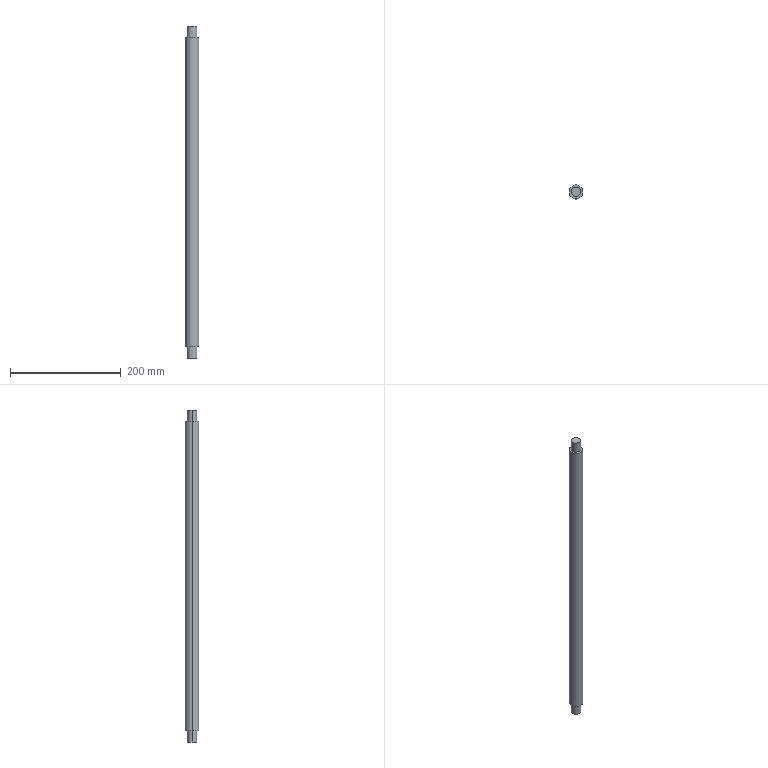Part | SolidWorks | features BaseBody 1 | 1 solid | 10 faces | box 25 x 25 x 600 mm | volume 283969 mm3 | cylinder 6 | plane 4 | commonest cylinder face diameters 17 x4 25 x2
STEP:
#1=CARTESIAN_POINT('',(8.5,0.,-560.));
#2=VERTEX_POINT('',#1);
#3=CARTESIAN_POINT('',(-8.5,0.,-560.));
#4=VERTEX_POINT('',#3);
#5=CARTESIAN_POINT('',(0.,0.,-560.));
#6=DIRECTION('',(0.,0.,1.));
#7=DIRECTION('',(-1.,0.,0.));
#8=AXIS2_PLACEMENT_3D('',#5,#6,#7);
#9=CIRCLE('',#8,8.5);
#10=EDGE_CURVE('',#2,#4,#9,.T.);
#11=ORIENTED_EDGE('',*,*,#10,.F.);
#12=CARTESIAN_POINT('',(8.5,0.,-580.));
#13=VERTEX_POINT('',#12);
#14=CARTESIAN_POINT('',(8.5,0.,-580.));
#15=DIRECTION('',(0.,0.,-1.));
#16=VECTOR('',#15,1000.);
#17=LINE('',#14,#16);
#18=EDGE_CURVE('',#2,#13,#17,.T.);
#19=ORIENTED_EDGE('',*,*,#18,.T.);
#20=CARTESIAN_POINT('',(-8.5,0.,-580.));
#21=VERTEX_POINT('',#20);
#22=CARTESIAN_POINT('',(0.,0.,-580.));
#23=DIRECTION('',(0.,0.,-1.));
#24=DIRECTION('',(-1.,0.,0.));
#25=AXIS2_PLACEMENT_3D('',#22,#23,#24);
#26=CIRCLE('',#25,8.5);
#27=EDGE_CURVE('',#21,#13,#26,.T.);
#28=ORIENTED_EDGE('',*,*,#27,.F.);
#29=CARTESIAN_POINT('',(-8.5,0.,-580.));
#30=DIRECTION('',(0.,0.,-1.));
#31=VECTOR('',#30,1000.);
#32=LINE('',#29,#31);
#33=EDGE_CURVE('',#4,#21,#32,.T.);
#34=ORIENTED_EDGE('',*,*,#33,.F.);
#35=EDGE_LOOP('',(#11,#19,#28,#34));
#36=FACE_OUTER_BOUND('',#35,.T.);
#37=CARTESIAN_POINT('',(0.,0.,-580.));
#38=DIRECTION('',(0.,0.,-1.));
#39=DIRECTION('',(-1.,0.,0.));
#40=AXIS2_PLACEMENT_3D('',#37,#38,#39);
#41=CYLINDRICAL_SURFACE('',#40,8.5);
#42=ADVANCED_FACE('',(#36),#41,.T.);
#43=CARTESIAN_POINT('',(8.5,0.,20.));
#44=VERTEX_POINT('',#43);
#45=CARTESIAN_POINT('',(-8.5,0.,20.));
#46=VERTEX_POINT('',#45);
#47=CARTESIAN_POINT('',(0.,0.,20.));
#48=DIRECTION('',(0.,0.,1.));
#49=DIRECTION('',(-1.,0.,0.));
#50=AXIS2_PLACEMENT_3D('',#47,#48,#49);
#51=CIRCLE('',#50,8.5);
#52=EDGE_CURVE('',#44,#46,#51,.T.);
#53=ORIENTED_EDGE('',*,*,#52,.F.);
#54=CARTESIAN_POINT('',(8.5,0.,0.));
#55=VERTEX_POINT('',#54);
#56=CARTESIAN_POINT('',(8.5,0.,0.));
#57=DIRECTION('',(0.,0.,-1.));
#58=VECTOR('',#57,1000.);
#59=LINE('',#56,#58);
#60=EDGE_CURVE('',#44,#55,#59,.T.);
#61=ORIENTED_EDGE('',*,*,#60,.T.);
#62=CARTESIAN_POINT('',(-8.5,0.,0.));
#63=VERTEX_POINT('',#62);
#64=CARTESIAN_POINT('',(0.,0.,0.));
#65=DIRECTION('',(0.,0.,-1.));
#66=DIRECTION('',(-1.,0.,0.));
#67=AXIS2_PLACEMENT_3D('',#64,#65,#66);
#68=CIRCLE('',#67,8.5);
#69=EDGE_CURVE('',#63,#55,#68,.T.);
#70=ORIENTED_EDGE('',*,*,#69,.F.);
#71=CARTESIAN_POINT('',(-8.5,0.,0.));
#72=DIRECTION('',(0.,0.,-1.));
#73=VECTOR('',#72,1000.);
#74=LINE('',#71,#73);
#75=EDGE_CURVE('',#46,#63,#74,.T.);
#76=ORIENTED_EDGE('',*,*,#75,.F.);
#77=EDGE_LOOP('',(#53,#61,#70,#76));
#78=FACE_OUTER_BOUND('',#77,.T.);
#79=CARTESIAN_POINT('',(0.,0.,0.));
#80=DIRECTION('',(0.,0.,-1.));
#81=DIRECTION('',(-1.,0.,0.));
#82=AXIS2_PLACEMENT_3D('',#79,#80,#81);
#83=CYLINDRICAL_SURFACE('',#82,8.5);
#84=ADVANCED_FACE('',(#78),#83,.T.);
#85=CARTESIAN_POINT('',(12.5,0.,-560.));
#86=VERTEX_POINT('',#85);
#87=CARTESIAN_POINT('',(-12.5,0.,-560.));
#88=VERTEX_POINT('',#87);
#89=CARTESIAN_POINT('',(0.,0.,-560.));
#90=DIRECTION('',(0.,0.,-1.));
#91=DIRECTION('',(-1.,0.,0.));
#92=AXIS2_PLACEMENT_3D('',#89,#90,#91);
#93=CIRCLE('',#92,12.5);
#94=EDGE_CURVE('',#86,#88,#93,.T.);
#95=ORIENTED_EDGE('',*,*,#94,.F.);
#96=CARTESIAN_POINT('',(12.5,0.,0.));
#97=VERTEX_POINT('',#96);
#98=CARTESIAN_POINT('',(12.5,0.,0.));
#99=DIRECTION('',(0.,0.,1.));
#100=VECTOR('',#99,1000.);
#101=LINE('',#98,#100);
#102=EDGE_CURVE('',#86,#97,#101,.T.);
#103=ORIENTED_EDGE('',*,*,#102,.T.);
#104=CARTESIAN_POINT('',(-12.5,0.,0.));
#105=VERTEX_POINT('',#104);
#106=CARTESIAN_POINT('',(0.,0.,0.));
#107=DIRECTION('',(0.,0.,-1.));
#108=DIRECTION('',(-1.,0.,0.));
#109=AXIS2_PLACEMENT_3D('',#106,#107,#108);
#110=CIRCLE('',#109,12.5);
#111=EDGE_CURVE('',#97,#105,#110,.T.);
#112=ORIENTED_EDGE('',*,*,#111,.T.);
#113=CARTESIAN_POINT('',(-12.5,0.,0.));
#114=DIRECTION('',(0.,0.,1.));
#115=VECTOR('',#114,1000.);
#116=LINE('',#113,#115);
#117=EDGE_CURVE('',#88,#105,#116,.T.);
#118=ORIENTED_EDGE('',*,*,#117,.F.);
#119=EDGE_LOOP('',(#95,#103,#112,#118));
#120=FACE_OUTER_BOUND('',#119,.T.);
#121=CARTESIAN_POINT('',(0.,0.,0.));
#122=DIRECTION('',(0.,0.,1.));
#123=DIRECTION('',(-1.,0.,0.));
#124=AXIS2_PLACEMENT_3D('',#121,#122,#123);
#125=CYLINDRICAL_SURFACE('',#124,12.5);
#126=ADVANCED_FACE('',(#120),#125,.T.);
#127=ORIENTED_EDGE('',*,*,#27,.T.);
#128=CARTESIAN_POINT('',(0.,0.,-580.));
#129=DIRECTION('',(0.,0.,-1.));
#130=DIRECTION('',(-1.,0.,0.));
#131=AXIS2_PLACEMENT_3D('',#128,#129,#130);
#132=CIRCLE('',#131,8.5);
#133=EDGE_CURVE('',#13,#21,#132,.T.);
#134=ORIENTED_EDGE('',*,*,#133,.T.);
#135=EDGE_LOOP('',(#127,#134));
#136=FACE_OUTER_BOUND('',#135,.T.);
#137=CARTESIAN_POINT('',(0.,0.,-580.));
#138=DIRECTION('',(0.,0.,1.));
#139=DIRECTION('',(1.,0.,0.));
#140=AXIS2_PLACEMENT_3D('',#137,#138,#139);
#141=PLANE('',#140);
#142=ADVANCED_FACE('',(#136),#141,.F.);
#143=CARTESIAN_POINT('',(0.,0.,20.));
#144=DIRECTION('',(0.,0.,1.));
#145=DIRECTION('',(-1.,0.,0.));
#146=AXIS2_PLACEMENT_3D('',#143,#144,#145);
#147=CIRCLE('',#146,8.5);
#148=EDGE_CURVE('',#46,#44,#147,.T.);
#149=ORIENTED_EDGE('',*,*,#148,.T.);
#150=ORIENTED_EDGE('',*,*,#52,.T.);
#151=EDGE_LOOP('',(#149,#150));
#152=FACE_OUTER_BOUND('',#151,.T.);
#153=CARTESIAN_POINT('',(0.,0.,20.));
#154=DIRECTION('',(0.,0.,1.));
#155=DIRECTION('',(1.,0.,0.));
#156=AXIS2_PLACEMENT_3D('',#153,#154,#155);
#157=PLANE('',#156);
#158=ADVANCED_FACE('',(#152),#157,.T.);
#159=CARTESIAN_POINT('',(0.,0.,-560.));
#160=DIRECTION('',(0.,0.,1.));
#161=DIRECTION('',(-1.,0.,0.));
#162=AXIS2_PLACEMENT_3D('',#159,#160,#161);
#163=CIRCLE('',#162,8.5);
#164=EDGE_CURVE('',#4,#2,#163,.T.);
#165=ORIENTED_EDGE('',*,*,#164,.T.);
#166=ORIENTED_EDGE('',*,*,#10,.T.);
#167=EDGE_LOOP('',(#165,#166));
#168=FACE_BOUND('',#167,.T.);
#169=CARTESIAN_POINT('',(0.,0.,-560.));
#170=DIRECTION('',(0.,0.,-1.));
#171=DIRECTION('',(-1.,0.,0.));
#172=AXIS2_PLACEMENT_3D('',#169,#170,#171);
#173=CIRCLE('',#172,12.5);
#174=EDGE_CURVE('',#88,#86,#173,.T.);
#175=ORIENTED_EDGE('',*,*,#174,.T.);
#176=ORIENTED_EDGE('',*,*,#94,.T.);
#177=EDGE_LOOP('',(#175,#176));
#178=FACE_OUTER_BOUND('',#177,.T.);
#179=CARTESIAN_POINT('',(0.,0.,-560.));
#180=DIRECTION('',(0.,0.,1.));
#181=DIRECTION('',(1.,0.,0.));
#182=AXIS2_PLACEMENT_3D('',#179,#180,#181);
#183=PLANE('',#182);
#184=ADVANCED_FACE('',(#168,#178),#183,.F.);
#185=ORIENTED_EDGE('',*,*,#69,.T.);
#186=CARTESIAN_POINT('',(0.,0.,0.));
#187=DIRECTION('',(0.,0.,-1.));
#188=DIRECTION('',(-1.,0.,0.));
#189=AXIS2_PLACEMENT_3D('',#186,#187,#188);
#190=CIRCLE('',#189,8.5);
#191=EDGE_CURVE('',#55,#63,#190,.T.);
#192=ORIENTED_EDGE('',*,*,#191,.T.);
#193=EDGE_LOOP('',(#185,#192));
#194=FACE_BOUND('',#193,.T.);
#195=CARTESIAN_POINT('',(0.,0.,0.));
#196=DIRECTION('',(0.,0.,-1.));
#197=DIRECTION('',(-1.,0.,0.));
#198=AXIS2_PLACEMENT_3D('',#195,#196,#197);
#199=CIRCLE('',#198,12.5);
#200=EDGE_CURVE('',#105,#97,#199,.T.);
#201=ORIENTED_EDGE('',*,*,#200,.F.);
#202=ORIENTED_EDGE('',*,*,#111,.F.);
#203=EDGE_LOOP('',(#201,#202));
#204=FACE_OUTER_BOUND('',#203,.T.);
#205=CARTESIAN_POINT('',(0.,0.,0.));
#206=DIRECTION('',(0.,0.,1.));
#207=DIRECTION('',(1.,0.,0.));
#208=AXIS2_PLACEMENT_3D('',#205,#206,#207);
#209=PLANE('',#208);
#210=ADVANCED_FACE('',(#194,#204),#209,.T.);
#211=ORIENTED_EDGE('',*,*,#102,.F.);
#212=ORIENTED_EDGE('',*,*,#174,.F.);
#213=ORIENTED_EDGE('',*,*,#117,.T.);
#214=ORIENTED_EDGE('',*,*,#200,.T.);
#215=EDGE_LOOP('',(#211,#212,#213,#214));
#216=FACE_OUTER_BOUND('',#215,.T.);
#217=CARTESIAN_POINT('',(0.,0.,0.));
#218=DIRECTION('',(0.,0.,1.));
#219=DIRECTION('',(-1.,0.,0.));
#220=AXIS2_PLACEMENT_3D('',#217,#218,#219);
#221=CYLINDRICAL_SURFACE('',#220,12.5);
#222=ADVANCED_FACE('',(#216),#221,.T.);
#223=ORIENTED_EDGE('',*,*,#60,.F.);
#224=ORIENTED_EDGE('',*,*,#148,.F.);
#225=ORIENTED_EDGE('',*,*,#75,.T.);
#226=ORIENTED_EDGE('',*,*,#191,.F.);
#227=EDGE_LOOP('',(#223,#224,#225,#226));
#228=FACE_OUTER_BOUND('',#227,.T.);
#229=CARTESIAN_POINT('',(0.,0.,0.));
#230=DIRECTION('',(0.,0.,-1.));
#231=DIRECTION('',(-1.,0.,0.));
#232=AXIS2_PLACEMENT_3D('',#229,#230,#231);
#233=CYLINDRICAL_SURFACE('',#232,8.5);
#234=ADVANCED_FACE('',(#228),#233,.T.);
#235=ORIENTED_EDGE('',*,*,#18,.F.);
#236=ORIENTED_EDGE('',*,*,#164,.F.);
#237=ORIENTED_EDGE('',*,*,#33,.T.);
#238=ORIENTED_EDGE('',*,*,#133,.F.);
#239=EDGE_LOOP('',(#235,#236,#237,#238));
#240=FACE_OUTER_BOUND('',#239,.T.);
#241=CARTESIAN_POINT('',(0.,0.,-580.));
#242=DIRECTION('',(0.,0.,-1.));
#243=DIRECTION('',(-1.,0.,0.));
#244=AXIS2_PLACEMENT_3D('',#241,#242,#243);
#245=CYLINDRICAL_SURFACE('',#244,8.5);
#246=ADVANCED_FACE('',(#240),#245,.T.);
#247=CLOSED_SHELL('',(#42,#84,#126,#142,#158,#184,#210,#222,#234,#246));
#248=MANIFOLD_SOLID_BREP('',#247);
#249=CARTESIAN_POINT('',(0.,0.,0.));
#250=DIRECTION('',(0.,0.,1.));
#251=DIRECTION('',(1.,0.,0.));
#252=AXIS2_PLACEMENT_3D('',#249,#250,#251);
#253=(LENGTH_UNIT()NAMED_UNIT(*)SI_UNIT(.MILLI.,.METRE.));
#254=UNCERTAINTY_MEASURE_WITH_UNIT(LENGTH_MEASURE(0.00001),#253,'','');
#255=(NAMED_UNIT(*)PLANE_ANGLE_UNIT()SI_UNIT($,.RADIAN.));
#256=(NAMED_UNIT(*)SI_UNIT($,.STERADIAN.)SOLID_ANGLE_UNIT());
#257=(GEOMETRIC_REPRESENTATION_CONTEXT(3)GLOBAL_UNCERTAINTY_ASSIGNED_CONTEXT((#254))GLOBAL_UNIT_ASSIGNED_CONTEXT((#253,#255,#256))REPRESENTATION_CONTEXT('',''));
#258=ADVANCED_BREP_SHAPE_REPRESENTATION('',(#248,#252),#257);